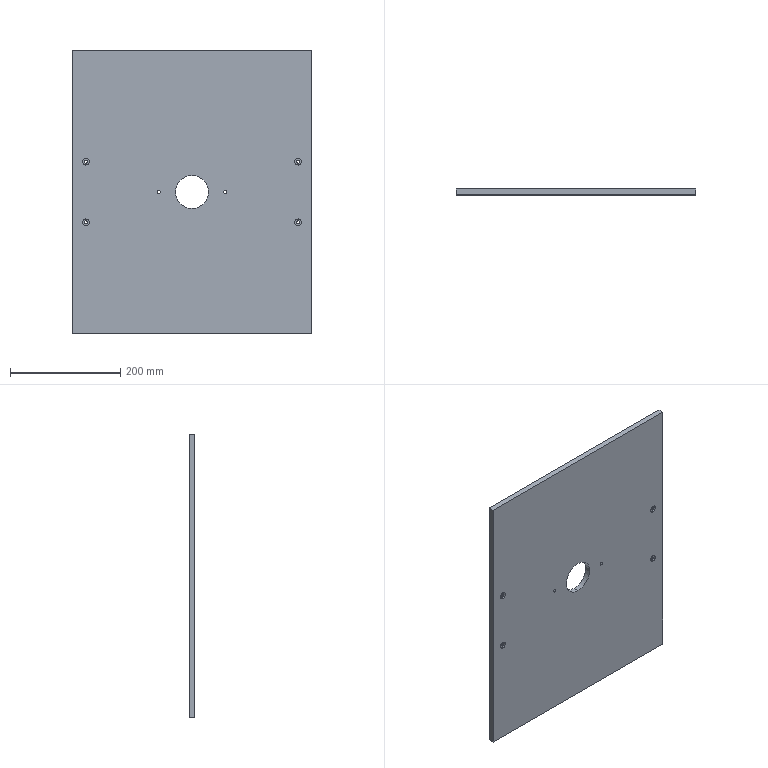Part | SolidWorks | features ICE 2, Extrusion 1, HoleWzd 1 | 1 solid | 40 faces | box 435 x 10 x 515 mm | volume 2209236 mm3 | cylinder 22 | plane 10 | cone 8 | commonest cylinder face diameters 5.5 x12 12.238 x8 60 x2
STEP:
#1=CARTESIAN_POINT('',(192.5,0.025,-48.881));
#2=VERTEX_POINT('',#1);
#3=CARTESIAN_POINT('',(192.5,0.025,-61.119));
#4=VERTEX_POINT('',#3);
#5=CARTESIAN_POINT('',(192.5,0.025,-55.));
#6=DIRECTION('',(0.,-1.,0.));
#7=DIRECTION('',(0.,0.,-1.));
#8=AXIS2_PLACEMENT_3D('',#5,#6,#7);
#9=CIRCLE('',#8,6.119);
#10=EDGE_CURVE('',#2,#4,#9,.T.);
#11=ORIENTED_EDGE('',*,*,#10,.F.);
#12=CARTESIAN_POINT('',(192.5,0.,-48.856));
#13=VERTEX_POINT('',#12);
#14=CARTESIAN_POINT('',(192.5,0.,-48.856));
#15=DIRECTION('',(0.,-0.7071,0.7071));
#16=VECTOR('',#15,1000.);
#17=LINE('',#14,#16);
#18=EDGE_CURVE('',#2,#13,#17,.T.);
#19=ORIENTED_EDGE('',*,*,#18,.T.);
#20=CARTESIAN_POINT('',(192.5,0.,-61.144));
#21=VERTEX_POINT('',#20);
#22=CARTESIAN_POINT('',(192.5,0.,-55.));
#23=DIRECTION('',(0.,-1.,0.));
#24=DIRECTION('',(0.,0.,-1.));
#25=AXIS2_PLACEMENT_3D('',#22,#23,#24);
#26=CIRCLE('',#25,6.144);
#27=EDGE_CURVE('',#13,#21,#26,.T.);
#28=ORIENTED_EDGE('',*,*,#27,.T.);
#29=CARTESIAN_POINT('',(192.5,0.,-61.144));
#30=DIRECTION('',(0.,-0.7071,-0.7071));
#31=VECTOR('',#30,1000.);
#32=LINE('',#29,#31);
#33=EDGE_CURVE('',#4,#21,#32,.T.);
#34=ORIENTED_EDGE('',*,*,#33,.F.);
#35=EDGE_LOOP('',(#11,#19,#28,#34));
#36=FACE_OUTER_BOUND('',#35,.T.);
#37=CARTESIAN_POINT('',(192.5,0.,-55.));
#38=DIRECTION('',(0.,-1.,0.));
#39=DIRECTION('',(0.,0.,-1.));
#40=AXIS2_PLACEMENT_3D('',#37,#38,#39);
#41=CONICAL_SURFACE('',#40,6.144,0.7854);
#42=ADVANCED_FACE('',(#36),#41,.F.);
#43=CARTESIAN_POINT('',(192.5,3.5,-48.881));
#44=VERTEX_POINT('',#43);
#45=CARTESIAN_POINT('',(192.5,3.5,-61.119));
#46=VERTEX_POINT('',#45);
#47=CARTESIAN_POINT('',(192.5,3.5,-55.));
#48=DIRECTION('',(0.,-1.,0.));
#49=DIRECTION('',(0.,0.,-1.));
#50=AXIS2_PLACEMENT_3D('',#47,#48,#49);
#51=CIRCLE('',#50,6.119);
#52=EDGE_CURVE('',#44,#46,#51,.T.);
#53=ORIENTED_EDGE('',*,*,#52,.F.);
#54=CARTESIAN_POINT('',(192.5,0.,-48.881));
#55=DIRECTION('',(0.,-1.,0.));
#56=VECTOR('',#55,1000.);
#57=LINE('',#54,#56);
#58=EDGE_CURVE('',#44,#2,#57,.T.);
#59=ORIENTED_EDGE('',*,*,#58,.T.);
#60=ORIENTED_EDGE('',*,*,#10,.T.);
#61=CARTESIAN_POINT('',(192.5,0.,-61.119));
#62=DIRECTION('',(0.,-1.,0.));
#63=VECTOR('',#62,1000.);
#64=LINE('',#61,#63);
#65=EDGE_CURVE('',#46,#4,#64,.T.);
#66=ORIENTED_EDGE('',*,*,#65,.F.);
#67=EDGE_LOOP('',(#53,#59,#60,#66));
#68=FACE_OUTER_BOUND('',#67,.T.);
#69=CARTESIAN_POINT('',(192.5,0.,-55.));
#70=DIRECTION('',(0.,-1.,0.));
#71=DIRECTION('',(0.,0.,-1.));
#72=AXIS2_PLACEMENT_3D('',#69,#70,#71);
#73=CYLINDRICAL_SURFACE('',#72,6.119);
#74=ADVANCED_FACE('',(#68),#73,.F.);
#75=CARTESIAN_POINT('',(192.5,10.,-52.25));
#76=VERTEX_POINT('',#75);
#77=CARTESIAN_POINT('',(192.5,10.,-57.75));
#78=VERTEX_POINT('',#77);
#79=CARTESIAN_POINT('',(192.5,10.,-55.));
#80=DIRECTION('',(0.,-1.,0.));
#81=DIRECTION('',(0.,0.,-1.));
#82=AXIS2_PLACEMENT_3D('',#79,#80,#81);
#83=CIRCLE('',#82,2.75);
#84=EDGE_CURVE('',#76,#78,#83,.T.);
#85=ORIENTED_EDGE('',*,*,#84,.F.);
#86=CARTESIAN_POINT('',(192.5,3.5,-52.25));
#87=VERTEX_POINT('',#86);
#88=CARTESIAN_POINT('',(192.5,0.,-52.25));
#89=DIRECTION('',(0.,-1.,0.));
#90=VECTOR('',#89,1000.);
#91=LINE('',#88,#90);
#92=EDGE_CURVE('',#76,#87,#91,.T.);
#93=ORIENTED_EDGE('',*,*,#92,.T.);
#94=CARTESIAN_POINT('',(192.5,3.5,-57.75));
#95=VERTEX_POINT('',#94);
#96=CARTESIAN_POINT('',(192.5,3.5,-55.));
#97=DIRECTION('',(0.,-1.,0.));
#98=DIRECTION('',(0.,0.,-1.));
#99=AXIS2_PLACEMENT_3D('',#96,#97,#98);
#100=CIRCLE('',#99,2.75);
#101=EDGE_CURVE('',#87,#95,#100,.T.);
#102=ORIENTED_EDGE('',*,*,#101,.T.);
#103=CARTESIAN_POINT('',(192.5,0.,-57.75));
#104=DIRECTION('',(0.,-1.,0.));
#105=VECTOR('',#104,1000.);
#106=LINE('',#103,#105);
#107=EDGE_CURVE('',#78,#95,#106,.T.);
#108=ORIENTED_EDGE('',*,*,#107,.F.);
#109=EDGE_LOOP('',(#85,#93,#102,#108));
#110=FACE_OUTER_BOUND('',#109,.T.);
#111=CARTESIAN_POINT('',(192.5,0.,-55.));
#112=DIRECTION('',(0.,-1.,0.));
#113=DIRECTION('',(0.,0.,-1.));
#114=AXIS2_PLACEMENT_3D('',#111,#112,#113);
#115=CYLINDRICAL_SURFACE('',#114,2.75);
#116=ADVANCED_FACE('',(#110),#115,.F.);
#117=CARTESIAN_POINT('',(192.5,0.025,61.119));
#118=VERTEX_POINT('',#117);
#119=CARTESIAN_POINT('',(192.5,0.025,48.881));
#120=VERTEX_POINT('',#119);
#121=CARTESIAN_POINT('',(192.5,0.025,55.));
#122=DIRECTION('',(0.,-1.,0.));
#123=DIRECTION('',(0.,0.,-1.));
#124=AXIS2_PLACEMENT_3D('',#121,#122,#123);
#125=CIRCLE('',#124,6.119);
#126=EDGE_CURVE('',#118,#120,#125,.T.);
#127=ORIENTED_EDGE('',*,*,#126,.F.);
#128=CARTESIAN_POINT('',(192.5,0.,61.144));
#129=VERTEX_POINT('',#128);
#130=CARTESIAN_POINT('',(192.5,0.,61.144));
#131=DIRECTION('',(0.,-0.7071,0.7071));
#132=VECTOR('',#131,1000.);
#133=LINE('',#130,#132);
#134=EDGE_CURVE('',#118,#129,#133,.T.);
#135=ORIENTED_EDGE('',*,*,#134,.T.);
#136=CARTESIAN_POINT('',(192.5,0.,48.856));
#137=VERTEX_POINT('',#136);
#138=CARTESIAN_POINT('',(192.5,0.,55.));
#139=DIRECTION('',(0.,-1.,0.));
#140=DIRECTION('',(0.,0.,-1.));
#141=AXIS2_PLACEMENT_3D('',#138,#139,#140);
#142=CIRCLE('',#141,6.144);
#143=EDGE_CURVE('',#129,#137,#142,.T.);
#144=ORIENTED_EDGE('',*,*,#143,.T.);
#145=CARTESIAN_POINT('',(192.5,0.,48.856));
#146=DIRECTION('',(0.,-0.7071,-0.7071));
#147=VECTOR('',#146,1000.);
#148=LINE('',#145,#147);
#149=EDGE_CURVE('',#120,#137,#148,.T.);
#150=ORIENTED_EDGE('',*,*,#149,.F.);
#151=EDGE_LOOP('',(#127,#135,#144,#150));
#152=FACE_OUTER_BOUND('',#151,.T.);
#153=CARTESIAN_POINT('',(192.5,0.,55.));
#154=DIRECTION('',(0.,-1.,0.));
#155=DIRECTION('',(0.,0.,-1.));
#156=AXIS2_PLACEMENT_3D('',#153,#154,#155);
#157=CONICAL_SURFACE('',#156,6.144,0.7854);
#158=ADVANCED_FACE('',(#152),#157,.F.);
#159=CARTESIAN_POINT('',(192.5,3.5,61.119));
#160=VERTEX_POINT('',#159);
#161=CARTESIAN_POINT('',(192.5,3.5,48.881));
#162=VERTEX_POINT('',#161);
#163=CARTESIAN_POINT('',(192.5,3.5,55.));
#164=DIRECTION('',(0.,-1.,0.));
#165=DIRECTION('',(0.,0.,-1.));
#166=AXIS2_PLACEMENT_3D('',#163,#164,#165);
#167=CIRCLE('',#166,6.119);
#168=EDGE_CURVE('',#160,#162,#167,.T.);
#169=ORIENTED_EDGE('',*,*,#168,.F.);
#170=CARTESIAN_POINT('',(192.5,0.,61.119));
#171=DIRECTION('',(0.,-1.,0.));
#172=VECTOR('',#171,1000.);
#173=LINE('',#170,#172);
#174=EDGE_CURVE('',#160,#118,#173,.T.);
#175=ORIENTED_EDGE('',*,*,#174,.T.);
#176=ORIENTED_EDGE('',*,*,#126,.T.);
#177=CARTESIAN_POINT('',(192.5,0.,48.881));
#178=DIRECTION('',(0.,-1.,0.));
#179=VECTOR('',#178,1000.);
#180=LINE('',#177,#179);
#181=EDGE_CURVE('',#162,#120,#180,.T.);
#182=ORIENTED_EDGE('',*,*,#181,.F.);
#183=EDGE_LOOP('',(#169,#175,#176,#182));
#184=FACE_OUTER_BOUND('',#183,.T.);
#185=CARTESIAN_POINT('',(192.5,0.,55.));
#186=DIRECTION('',(0.,-1.,0.));
#187=DIRECTION('',(0.,0.,-1.));
#188=AXIS2_PLACEMENT_3D('',#185,#186,#187);
#189=CYLINDRICAL_SURFACE('',#188,6.119);
#190=ADVANCED_FACE('',(#184),#189,.F.);
#191=CARTESIAN_POINT('',(192.5,10.,57.75));
#192=VERTEX_POINT('',#191);
#193=CARTESIAN_POINT('',(192.5,10.,52.25));
#194=VERTEX_POINT('',#193);
#195=CARTESIAN_POINT('',(192.5,10.,55.));
#196=DIRECTION('',(0.,-1.,0.));
#197=DIRECTION('',(0.,0.,-1.));
#198=AXIS2_PLACEMENT_3D('',#195,#196,#197);
#199=CIRCLE('',#198,2.75);
#200=EDGE_CURVE('',#192,#194,#199,.T.);
#201=ORIENTED_EDGE('',*,*,#200,.F.);
#202=CARTESIAN_POINT('',(192.5,3.5,57.75));
#203=VERTEX_POINT('',#202);
#204=CARTESIAN_POINT('',(192.5,0.,57.75));
#205=DIRECTION('',(0.,-1.,0.));
#206=VECTOR('',#205,1000.);
#207=LINE('',#204,#206);
#208=EDGE_CURVE('',#192,#203,#207,.T.);
#209=ORIENTED_EDGE('',*,*,#208,.T.);
#210=CARTESIAN_POINT('',(192.5,3.5,52.25));
#211=VERTEX_POINT('',#210);
#212=CARTESIAN_POINT('',(192.5,3.5,55.));
#213=DIRECTION('',(0.,-1.,0.));
#214=DIRECTION('',(0.,0.,-1.));
#215=AXIS2_PLACEMENT_3D('',#212,#213,#214);
#216=CIRCLE('',#215,2.75);
#217=EDGE_CURVE('',#203,#211,#216,.T.);
#218=ORIENTED_EDGE('',*,*,#217,.T.);
#219=CARTESIAN_POINT('',(192.5,0.,52.25));
#220=DIRECTION('',(0.,-1.,0.));
#221=VECTOR('',#220,1000.);
#222=LINE('',#219,#221);
#223=EDGE_CURVE('',#194,#211,#222,.T.);
#224=ORIENTED_EDGE('',*,*,#223,.F.);
#225=EDGE_LOOP('',(#201,#209,#218,#224));
#226=FACE_OUTER_BOUND('',#225,.T.);
#227=CARTESIAN_POINT('',(192.5,0.,55.));
#228=DIRECTION('',(0.,-1.,0.));
#229=DIRECTION('',(0.,0.,-1.));
#230=AXIS2_PLACEMENT_3D('',#227,#228,#229);
#231=CYLINDRICAL_SURFACE('',#230,2.75);
#232=ADVANCED_FACE('',(#226),#231,.F.);
#233=CARTESIAN_POINT('',(-192.5,0.025,61.119));
#234=VERTEX_POINT('',#233);
#235=CARTESIAN_POINT('',(-192.5,0.025,48.881));
#236=VERTEX_POINT('',#235);
#237=CARTESIAN_POINT('',(-192.5,0.025,55.));
#238=DIRECTION('',(0.,-1.,0.));
#239=DIRECTION('',(0.,0.,-1.));
#240=AXIS2_PLACEMENT_3D('',#237,#238,#239);
#241=CIRCLE('',#240,6.119);
#242=EDGE_CURVE('',#234,#236,#241,.T.);
#243=ORIENTED_EDGE('',*,*,#242,.F.);
#244=CARTESIAN_POINT('',(-192.5,0.,61.144));
#245=VERTEX_POINT('',#244);
#246=CARTESIAN_POINT('',(-192.5,0.,61.144));
#247=DIRECTION('',(0.,-0.7071,0.7071));
#248=VECTOR('',#247,1000.);
#249=LINE('',#246,#248);
#250=EDGE_CURVE('',#234,#245,#249,.T.);
#251=ORIENTED_EDGE('',*,*,#250,.T.);
#252=CARTESIAN_POINT('',(-192.5,0.,48.856));
#253=VERTEX_POINT('',#252);
#254=CARTESIAN_POINT('',(-192.5,0.,55.));
#255=DIRECTION('',(0.,-1.,0.));
#256=DIRECTION('',(0.,0.,-1.));
#257=AXIS2_PLACEMENT_3D('',#254,#255,#256);
#258=CIRCLE('',#257,6.144);
#259=EDGE_CURVE('',#245,#253,#258,.T.);
#260=ORIENTED_EDGE('',*,*,#259,.T.);
#261=CARTESIAN_POINT('',(-192.5,0.,48.856));
#262=DIRECTION('',(0.,-0.7071,-0.7071));
#263=VECTOR('',#262,1000.);
#264=LINE('',#261,#263);
#265=EDGE_CURVE('',#236,#253,#264,.T.);
#266=ORIENTED_EDGE('',*,*,#265,.F.);
#267=EDGE_LOOP('',(#243,#251,#260,#266));
#268=FACE_OUTER_BOUND('',#267,.T.);
#269=CARTESIAN_POINT('',(-192.5,0.,55.));
#270=DIRECTION('',(0.,-1.,0.));
#271=DIRECTION('',(0.,0.,-1.));
#272=AXIS2_PLACEMENT_3D('',#269,#270,#271);
#273=CONICAL_SURFACE('',#272,6.144,0.7854);
#274=ADVANCED_FACE('',(#268),#273,.F.);
#275=CARTESIAN_POINT('',(-192.5,3.5,61.119));
#276=VERTEX_POINT('',#275);
#277=CARTESIAN_POINT('',(-192.5,3.5,48.881));
#278=VERTEX_POINT('',#277);
#279=CARTESIAN_POINT('',(-192.5,3.5,55.));
#280=DIRECTION('',(0.,-1.,0.));
#281=DIRECTION('',(0.,0.,-1.));
#282=AXIS2_PLACEMENT_3D('',#279,#280,#281);
#283=CIRCLE('',#282,6.119);
#284=EDGE_CURVE('',#276,#278,#283,.T.);
#285=ORIENTED_EDGE('',*,*,#284,.F.);
#286=CARTESIAN_POINT('',(-192.5,0.,61.119));
#287=DIRECTION('',(0.,-1.,0.));
#288=VECTOR('',#287,1000.);
#289=LINE('',#286,#288);
#290=EDGE_CURVE('',#276,#234,#289,.T.);
#291=ORIENTED_EDGE('',*,*,#290,.T.);
#292=ORIENTED_EDGE('',*,*,#242,.T.);
#293=CARTESIAN_POINT('',(-192.5,0.,48.881));
#294=DIRECTION('',(0.,-1.,0.));
#295=VECTOR('',#294,1000.);
#296=LINE('',#293,#295);
#297=EDGE_CURVE('',#278,#236,#296,.T.);
#298=ORIENTED_EDGE('',*,*,#297,.F.);
#299=EDGE_LOOP('',(#285,#291,#292,#298));
#300=FACE_OUTER_BOUND('',#299,.T.);
#301=CARTESIAN_POINT('',(-192.5,0.,55.));
#302=DIRECTION('',(0.,-1.,0.));
#303=DIRECTION('',(0.,0.,-1.));
#304=AXIS2_PLACEMENT_3D('',#301,#302,#303);
#305=CYLINDRICAL_SURFACE('',#304,6.119);
#306=ADVANCED_FACE('',(#300),#305,.F.);
#307=CARTESIAN_POINT('',(-192.5,10.,57.75));
#308=VERTEX_POINT('',#307);
#309=CARTESIAN_POINT('',(-192.5,10.,52.25));
#310=VERTEX_POINT('',#309);
#311=CARTESIAN_POINT('',(-192.5,10.,55.));
#312=DIRECTION('',(0.,-1.,0.));
#313=DIRECTION('',(0.,0.,-1.));
#314=AXIS2_PLACEMENT_3D('',#311,#312,#313);
#315=CIRCLE('',#314,2.75);
#316=EDGE_CURVE('',#308,#310,#315,.T.);
#317=ORIENTED_EDGE('',*,*,#316,.F.);
#318=CARTESIAN_POINT('',(-192.5,3.5,57.75));
#319=VERTEX_POINT('',#318);
#320=CARTESIAN_POINT('',(-192.5,0.,57.75));
#321=DIRECTION('',(0.,-1.,0.));
#322=VECTOR('',#321,1000.);
#323=LINE('',#320,#322);
#324=EDGE_CURVE('',#308,#319,#323,.T.);
#325=ORIENTED_EDGE('',*,*,#324,.T.);
#326=CARTESIAN_POINT('',(-192.5,3.5,52.25));
#327=VERTEX_POINT('',#326);
#328=CARTESIAN_POINT('',(-192.5,3.5,55.));
#329=DIRECTION('',(0.,-1.,0.));
#330=DIRECTION('',(0.,0.,-1.));
#331=AXIS2_PLACEMENT_3D('',#328,#329,#330);
#332=CIRCLE('',#331,2.75);
#333=EDGE_CURVE('',#319,#327,#332,.T.);
#334=ORIENTED_EDGE('',*,*,#333,.T.);
#335=CARTESIAN_POINT('',(-192.5,0.,52.25));
#336=DIRECTION('',(0.,-1.,0.));
#337=VECTOR('',#336,1000.);
#338=LINE('',#335,#337);
#339=EDGE_CURVE('',#310,#327,#338,.T.);
#340=ORIENTED_EDGE('',*,*,#339,.F.);
#341=EDGE_LOOP('',(#317,#325,#334,#340));
#342=FACE_OUTER_BOUND('',#341,.T.);
#343=CARTESIAN_POINT('',(-192.5,0.,55.));
#344=DIRECTION('',(0.,-1.,0.));
#345=DIRECTION('',(0.,0.,-1.));
#346=AXIS2_PLACEMENT_3D('',#343,#344,#345);
#347=CYLINDRICAL_SURFACE('',#346,2.75);
#348=ADVANCED_FACE('',(#342),#347,.F.);
#349=CARTESIAN_POINT('',(-192.5,0.025,-48.881));
#350=VERTEX_POINT('',#349);
#351=CARTESIAN_POINT('',(-192.5,0.025,-61.119));
#352=VERTEX_POINT('',#351);
#353=CARTESIAN_POINT('',(-192.5,0.025,-55.));
#354=DIRECTION('',(0.,-1.,0.));
#355=DIRECTION('',(0.,0.,-1.));
#356=AXIS2_PLACEMENT_3D('',#353,#354,#355);
#357=CIRCLE('',#356,6.119);
#358=EDGE_CURVE('',#350,#352,#357,.T.);
#359=ORIENTED_EDGE('',*,*,#358,.F.);
#360=CARTESIAN_POINT('',(-192.5,0.,-48.856));
#361=VERTEX_POINT('',#360);
#362=CARTESIAN_POINT('',(-192.5,0.,-48.856));
#363=DIRECTION('',(0.,-0.7071,0.7071));
#364=VECTOR('',#363,1000.);
#365=LINE('',#362,#364);
#366=EDGE_CURVE('',#350,#361,#365,.T.);
#367=ORIENTED_EDGE('',*,*,#366,.T.);
#368=CARTESIAN_POINT('',(-192.5,0.,-61.144));
#369=VERTEX_POINT('',#368);
#370=CARTESIAN_POINT('',(-192.5,0.,-55.));
#371=DIRECTION('',(0.,-1.,0.));
#372=DIRECTION('',(0.,0.,-1.));
#373=AXIS2_PLACEMENT_3D('',#370,#371,#372);
#374=CIRCLE('',#373,6.144);
#375=EDGE_CURVE('',#361,#369,#374,.T.);
#376=ORIENTED_EDGE('',*,*,#375,.T.);
#377=CARTESIAN_POINT('',(-192.5,0.,-61.144));
#378=DIRECTION('',(0.,-0.7071,-0.7071));
#379=VECTOR('',#378,1000.);
#380=LINE('',#377,#379);
#381=EDGE_CURVE('',#352,#369,#380,.T.);
#382=ORIENTED_EDGE('',*,*,#381,.F.);
#383=EDGE_LOOP('',(#359,#367,#376,#382));
#384=FACE_OUTER_BOUND('',#383,.T.);
#385=CARTESIAN_POINT('',(-192.5,0.,-55.));
#386=DIRECTION('',(0.,-1.,0.));
#387=DIRECTION('',(0.,0.,-1.));
#388=AXIS2_PLACEMENT_3D('',#385,#386,#387);
#389=CONICAL_SURFACE('',#388,6.144,0.7854);
#390=ADVANCED_FACE('',(#384),#389,.F.);
#391=CARTESIAN_POINT('',(-192.5,3.5,-48.881));
#392=VERTEX_POINT('',#391);
#393=CARTESIAN_POINT('',(-192.5,3.5,-61.119));
#394=VERTEX_POINT('',#393);
#395=CARTESIAN_POINT('',(-192.5,3.5,-55.));
#396=DIRECTION('',(0.,-1.,0.));
#397=DIRECTION('',(0.,0.,-1.));
#398=AXIS2_PLACEMENT_3D('',#395,#396,#397);
#399=CIRCLE('',#398,6.119);
#400=EDGE_CURVE('',#392,#394,#399,.T.);
#401=ORIENTED_EDGE('',*,*,#400,.F.);
#402=CARTESIAN_POINT('',(-192.5,0.,-48.881));
#403=DIRECTION('',(0.,-1.,0.));
#404=VECTOR('',#403,1000.);
#405=LINE('',#402,#404);
#406=EDGE_CURVE('',#392,#350,#405,.T.);
#407=ORIENTED_EDGE('',*,*,#406,.T.);
#408=ORIENTED_EDGE('',*,*,#358,.T.);
#409=CARTESIAN_POINT('',(-192.5,0.,-61.119));
#410=DIRECTION('',(0.,-1.,0.));
#411=VECTOR('',#410,1000.);
#412=LINE('',#409,#411);
#413=EDGE_CURVE('',#394,#352,#412,.T.);
#414=ORIENTED_EDGE('',*,*,#413,.F.);
#415=EDGE_LOOP('',(#401,#407,#408,#414));
#416=FACE_OUTER_BOUND('',#415,.T.);
#417=CARTESIAN_POINT('',(-192.5,0.,-55.));
#418=DIRECTION('',(0.,-1.,0.));
#419=DIRECTION('',(0.,0.,-1.));
#420=AXIS2_PLACEMENT_3D('',#417,#418,#419);
#421=CYLINDRICAL_SURFACE('',#420,6.119);
#422=ADVANCED_FACE('',(#416),#421,.F.);
#423=CARTESIAN_POINT('',(-192.5,10.,-52.25));
#424=VERTEX_POINT('',#423);
#425=CARTESIAN_POINT('',(-192.5,10.,-57.75));
#426=VERTEX_POINT('',#425);
#427=CARTESIAN_POINT('',(-192.5,10.,-55.));
#428=DIRECTION('',(0.,-1.,0.));
#429=DIRECTION('',(0.,0.,-1.));
#430=AXIS2_PLACEMENT_3D('',#427,#428,#429);
#431=CIRCLE('',#430,2.75);
#432=EDGE_CURVE('',#424,#426,#431,.T.);
#433=ORIENTED_EDGE('',*,*,#432,.F.);
#434=CARTESIAN_POINT('',(-192.5,3.5,-52.25));
#435=VERTEX_POINT('',#434);
#436=CARTESIAN_POINT('',(-192.5,0.,-52.25));
#437=DIRECTION('',(0.,-1.,0.));
#438=VECTOR('',#437,1000.);
#439=LINE('',#436,#438);
#440=EDGE_CURVE('',#424,#435,#439,.T.);
#441=ORIENTED_EDGE('',*,*,#440,.T.);
#442=CARTESIAN_POINT('',(-192.5,3.5,-57.75));
#443=VERTEX_POINT('',#442);
#444=CARTESIAN_POINT('',(-192.5,3.5,-55.));
#445=DIRECTION('',(0.,-1.,0.));
#446=DIRECTION('',(0.,0.,-1.));
#447=AXIS2_PLACEMENT_3D('',#444,#445,#446);
#448=CIRCLE('',#447,2.75);
#449=EDGE_CURVE('',#435,#443,#448,.T.);
#450=ORIENTED_EDGE('',*,*,#449,.T.);
#451=CARTESIAN_POINT('',(-192.5,0.,-57.75));
#452=DIRECTION('',(0.,-1.,0.));
#453=VECTOR('',#452,1000.);
#454=LINE('',#451,#453);
#455=EDGE_CURVE('',#426,#443,#454,.T.);
#456=ORIENTED_EDGE('',*,*,#455,.F.);
#457=EDGE_LOOP('',(#433,#441,#450,#456));
#458=FACE_OUTER_BOUND('',#457,.T.);
#459=CARTESIAN_POINT('',(-192.5,0.,-55.));
#460=DIRECTION('',(0.,-1.,0.));
#461=DIRECTION('',(0.,0.,-1.));
#462=AXIS2_PLACEMENT_3D('',#459,#460,#461);
#463=CYLINDRICAL_SURFACE('',#462,2.75);
#464=ADVANCED_FACE('',(#458),#463,.F.);
#465=CARTESIAN_POINT('',(-60.,0.,-2.75));
#466=VERTEX_POINT('',#465);
#467=CARTESIAN_POINT('',(-60.,0.,2.75));
#468=VERTEX_POINT('',#467);
#469=CARTESIAN_POINT('',(-60.,0.,0.));
#470=DIRECTION('',(0.,1.,0.));
#471=DIRECTION('',(0.,0.,1.));
#472=AXIS2_PLACEMENT_3D('',#469,#470,#471);
#473=CIRCLE('',#472,2.75);
#474=EDGE_CURVE('',#466,#468,#473,.T.);
#475=ORIENTED_EDGE('',*,*,#474,.F.);
#476=CARTESIAN_POINT('',(-60.,10.,-2.75));
#477=VERTEX_POINT('',#476);
#478=CARTESIAN_POINT('',(-60.,0.,-2.75));
#479=DIRECTION('',(0.,1.,0.));
#480=VECTOR('',#479,1000.);
#481=LINE('',#478,#480);
#482=EDGE_CURVE('',#466,#477,#481,.T.);
#483=ORIENTED_EDGE('',*,*,#482,.T.);
#484=CARTESIAN_POINT('',(-60.,10.,2.75));
#485=VERTEX_POINT('',#484);
#486=CARTESIAN_POINT('',(-60.,10.,0.));
#487=DIRECTION('',(0.,1.,0.));
#488=DIRECTION('',(0.,0.,1.));
#489=AXIS2_PLACEMENT_3D('',#486,#487,#488);
#490=CIRCLE('',#489,2.75);
#491=EDGE_CURVE('',#477,#485,#490,.T.);
#492=ORIENTED_EDGE('',*,*,#491,.T.);
#493=CARTESIAN_POINT('',(-60.,0.,2.75));
#494=DIRECTION('',(0.,1.,0.));
#495=VECTOR('',#494,1000.);
#496=LINE('',#493,#495);
#497=EDGE_CURVE('',#468,#485,#496,.T.);
#498=ORIENTED_EDGE('',*,*,#497,.F.);
#499=EDGE_LOOP('',(#475,#483,#492,#498));
#500=FACE_OUTER_BOUND('',#499,.T.);
#501=CARTESIAN_POINT('',(-60.,0.,0.));
#502=DIRECTION('',(0.,1.,0.));
#503=DIRECTION('',(0.,0.,1.));
#504=AXIS2_PLACEMENT_3D('',#501,#502,#503);
#505=CYLINDRICAL_SURFACE('',#504,2.75);
#506=ADVANCED_FACE('',(#500),#505,.F.);
#507=CARTESIAN_POINT('',(60.,0.,-2.75));
#508=VERTEX_POINT('',#507);
#509=CARTESIAN_POINT('',(60.,0.,2.75));
#510=VERTEX_POINT('',#509);
#511=CARTESIAN_POINT('',(60.,0.,0.));
#512=DIRECTION('',(0.,1.,0.));
#513=DIRECTION('',(0.,0.,1.));
#514=AXIS2_PLACEMENT_3D('',#511,#512,#513);
#515=CIRCLE('',#514,2.75);
#516=EDGE_CURVE('',#508,#510,#515,.T.);
#517=ORIENTED_EDGE('',*,*,#516,.F.);
#518=CARTESIAN_POINT('',(60.,10.,-2.75));
#519=VERTEX_POINT('',#518);
#520=CARTESIAN_POINT('',(60.,0.,-2.75));
#521=DIRECTION('',(0.,1.,0.));
#522=VECTOR('',#521,1000.);
#523=LINE('',#520,#522);
#524=EDGE_CURVE('',#508,#519,#523,.T.);
#525=ORIENTED_EDGE('',*,*,#524,.T.);
#526=CARTESIAN_POINT('',(60.,10.,2.75));
#527=VERTEX_POINT('',#526);
#528=CARTESIAN_POINT('',(60.,10.,0.));
#529=DIRECTION('',(0.,1.,0.));
#530=DIRECTION('',(0.,0.,1.));
#531=AXIS2_PLACEMENT_3D('',#528,#529,#530);
#532=CIRCLE('',#531,2.75);
#533=EDGE_CURVE('',#519,#527,#532,.T.);
#534=ORIENTED_EDGE('',*,*,#533,.T.);
#535=CARTESIAN_POINT('',(60.,0.,2.75));
#536=DIRECTION('',(0.,1.,0.));
#537=VECTOR('',#536,1000.);
#538=LINE('',#535,#537);
#539=EDGE_CURVE('',#510,#527,#538,.T.);
#540=ORIENTED_EDGE('',*,*,#539,.F.);
#541=EDGE_LOOP('',(#517,#525,#534,#540));
#542=FACE_OUTER_BOUND('',#541,.T.);
#543=CARTESIAN_POINT('',(60.,0.,0.));
#544=DIRECTION('',(0.,1.,0.));
#545=DIRECTION('',(0.,0.,1.));
#546=AXIS2_PLACEMENT_3D('',#543,#544,#545);
#547=CYLINDRICAL_SURFACE('',#546,2.75);
#548=ADVANCED_FACE('',(#542),#547,.F.);
#549=CARTESIAN_POINT('',(0.,0.,-30.));
#550=VERTEX_POINT('',#549);
#551=CARTESIAN_POINT('',(0.,0.,30.));
#552=VERTEX_POINT('',#551);
#553=CARTESIAN_POINT('',(0.,0.,0.));
#554=DIRECTION('',(0.,1.,0.));
#555=DIRECTION('',(0.,0.,1.));
#556=AXIS2_PLACEMENT_3D('',#553,#554,#555);
#557=CIRCLE('',#556,30.);
#558=EDGE_CURVE('',#550,#552,#557,.T.);
#559=ORIENTED_EDGE('',*,*,#558,.F.);
#560=CARTESIAN_POINT('',(0.,10.,-30.));
#561=VERTEX_POINT('',#560);
#562=CARTESIAN_POINT('',(0.,0.,-30.));
#563=DIRECTION('',(0.,1.,0.));
#564=VECTOR('',#563,1000.);
#565=LINE('',#562,#564);
#566=EDGE_CURVE('',#550,#561,#565,.T.);
#567=ORIENTED_EDGE('',*,*,#566,.T.);
#568=CARTESIAN_POINT('',(0.,10.,30.));
#569=VERTEX_POINT('',#568);
#570=CARTESIAN_POINT('',(0.,10.,0.));
#571=DIRECTION('',(0.,1.,0.));
#572=DIRECTION('',(0.,0.,1.));
#573=AXIS2_PLACEMENT_3D('',#570,#571,#572);
#574=CIRCLE('',#573,30.);
#575=EDGE_CURVE('',#561,#569,#574,.T.);
#576=ORIENTED_EDGE('',*,*,#575,.T.);
#577=CARTESIAN_POINT('',(0.,0.,30.));
#578=DIRECTION('',(0.,1.,0.));
#579=VECTOR('',#578,1000.);
#580=LINE('',#577,#579);
#581=EDGE_CURVE('',#552,#569,#580,.T.);
#582=ORIENTED_EDGE('',*,*,#581,.F.);
#583=EDGE_LOOP('',(#559,#567,#576,#582));
#584=FACE_OUTER_BOUND('',#583,.T.);
#585=CARTESIAN_POINT('',(0.,0.,0.));
#586=DIRECTION('',(0.,1.,0.));
#587=DIRECTION('',(0.,0.,1.));
#588=AXIS2_PLACEMENT_3D('',#585,#586,#587);
#589=CYLINDRICAL_SURFACE('',#588,30.);
#590=ADVANCED_FACE('',(#584),#589,.F.);
#591=CARTESIAN_POINT('',(217.5,0.,257.5));
#592=VERTEX_POINT('',#591);
#593=CARTESIAN_POINT('',(217.5,0.,-257.5));
#594=VERTEX_POINT('',#593);
#595=CARTESIAN_POINT('',(217.5,0.,257.5));
#596=DIRECTION('',(0.,0.,-1.));
#597=VECTOR('',#596,1000.);
#598=LINE('',#595,#597);
#599=EDGE_CURVE('',#592,#594,#598,.T.);
#600=ORIENTED_EDGE('',*,*,#599,.T.);
#601=CARTESIAN_POINT('',(217.5,10.,-257.5));
#602=VERTEX_POINT('',#601);
#603=CARTESIAN_POINT('',(217.5,10.,-257.5));
#604=DIRECTION('',(0.,-1.,0.));
#605=VECTOR('',#604,1000.);
#606=LINE('',#603,#605);
#607=EDGE_CURVE('',#602,#594,#606,.T.);
#608=ORIENTED_EDGE('',*,*,#607,.F.);
#609=CARTESIAN_POINT('',(217.5,10.,257.5));
#610=VERTEX_POINT('',#609);
#611=CARTESIAN_POINT('',(217.5,10.,257.5));
#612=DIRECTION('',(0.,0.,-1.));
#613=VECTOR('',#612,1000.);
#614=LINE('',#611,#613);
#615=EDGE_CURVE('',#610,#602,#614,.T.);
#616=ORIENTED_EDGE('',*,*,#615,.F.);
#617=CARTESIAN_POINT('',(217.5,10.,257.5));
#618=DIRECTION('',(0.,-1.,0.));
#619=VECTOR('',#618,1000.);
#620=LINE('',#617,#619);
#621=EDGE_CURVE('',#610,#592,#620,.T.);
#622=ORIENTED_EDGE('',*,*,#621,.T.);
#623=EDGE_LOOP('',(#600,#608,#616,#622));
#624=FACE_OUTER_BOUND('',#623,.T.);
#625=CARTESIAN_POINT('',(217.5,10.,257.5));
#626=DIRECTION('',(-1.,0.,0.));
#627=DIRECTION('',(0.,0.,1.));
#628=AXIS2_PLACEMENT_3D('',#625,#626,#627);
#629=PLANE('',#628);
#630=ADVANCED_FACE('',(#624),#629,.F.);
#631=CARTESIAN_POINT('',(-217.5,0.,-257.5));
#632=VERTEX_POINT('',#631);
#633=CARTESIAN_POINT('',(-217.5,0.,-257.5));
#634=DIRECTION('',(-1.,0.,0.));
#635=VECTOR('',#634,1000.);
#636=LINE('',#633,#635);
#637=EDGE_CURVE('',#594,#632,#636,.T.);
#638=ORIENTED_EDGE('',*,*,#637,.T.);
#639=CARTESIAN_POINT('',(-217.5,10.,-257.5));
#640=VERTEX_POINT('',#639);
#641=CARTESIAN_POINT('',(-217.5,10.,-257.5));
#642=DIRECTION('',(0.,-1.,0.));
#643=VECTOR('',#642,1000.);
#644=LINE('',#641,#643);
#645=EDGE_CURVE('',#640,#632,#644,.T.);
#646=ORIENTED_EDGE('',*,*,#645,.F.);
#647=CARTESIAN_POINT('',(-217.5,10.,-257.5));
#648=DIRECTION('',(-1.,0.,0.));
#649=VECTOR('',#648,1000.);
#650=LINE('',#647,#649);
#651=EDGE_CURVE('',#602,#640,#650,.T.);
#652=ORIENTED_EDGE('',*,*,#651,.F.);
#653=ORIENTED_EDGE('',*,*,#607,.T.);
#654=EDGE_LOOP('',(#638,#646,#652,#653));
#655=FACE_OUTER_BOUND('',#654,.T.);
#656=CARTESIAN_POINT('',(-217.5,10.,-257.5));
#657=DIRECTION('',(0.,0.,1.));
#658=DIRECTION('',(1.,0.,0.));
#659=AXIS2_PLACEMENT_3D('',#656,#657,#658);
#660=PLANE('',#659);
#661=ADVANCED_FACE('',(#655),#660,.F.);
#662=CARTESIAN_POINT('',(-217.5,0.,257.5));
#663=VERTEX_POINT('',#662);
#664=CARTESIAN_POINT('',(-217.5,0.,257.5));
#665=DIRECTION('',(0.,0.,1.));
#666=VECTOR('',#665,1000.);
#667=LINE('',#664,#666);
#668=EDGE_CURVE('',#632,#663,#667,.T.);
#669=ORIENTED_EDGE('',*,*,#668,.T.);
#670=CARTESIAN_POINT('',(-217.5,10.,257.5));
#671=VERTEX_POINT('',#670);
#672=CARTESIAN_POINT('',(-217.5,10.,257.5));
#673=DIRECTION('',(0.,-1.,0.));
#674=VECTOR('',#673,1000.);
#675=LINE('',#672,#674);
#676=EDGE_CURVE('',#671,#663,#675,.T.);
#677=ORIENTED_EDGE('',*,*,#676,.F.);
#678=CARTESIAN_POINT('',(-217.5,10.,257.5));
#679=DIRECTION('',(0.,0.,1.));
#680=VECTOR('',#679,1000.);
#681=LINE('',#678,#680);
#682=EDGE_CURVE('',#640,#671,#681,.T.);
#683=ORIENTED_EDGE('',*,*,#682,.F.);
#684=ORIENTED_EDGE('',*,*,#645,.T.);
#685=EDGE_LOOP('',(#669,#677,#683,#684));
#686=FACE_OUTER_BOUND('',#685,.T.);
#687=CARTESIAN_POINT('',(-217.5,10.,257.5));
#688=DIRECTION('',(1.,0.,0.));
#689=DIRECTION('',(0.,0.,-1.));
#690=AXIS2_PLACEMENT_3D('',#687,#688,#689);
#691=PLANE('',#690);
#692=ADVANCED_FACE('',(#686),#691,.F.);
#693=CARTESIAN_POINT('',(-217.5,0.,257.5));
#694=DIRECTION('',(1.,0.,0.));
#695=VECTOR('',#694,1000.);
#696=LINE('',#693,#695);
#697=EDGE_CURVE('',#663,#592,#696,.T.);
#698=ORIENTED_EDGE('',*,*,#697,.T.);
#699=ORIENTED_EDGE('',*,*,#621,.F.);
#700=CARTESIAN_POINT('',(-217.5,10.,257.5));
#701=DIRECTION('',(1.,0.,0.));
#702=VECTOR('',#701,1000.);
#703=LINE('',#700,#702);
#704=EDGE_CURVE('',#671,#610,#703,.T.);
#705=ORIENTED_EDGE('',*,*,#704,.F.);
#706=ORIENTED_EDGE('',*,*,#676,.T.);
#707=EDGE_LOOP('',(#698,#699,#705,#706));
#708=FACE_OUTER_BOUND('',#707,.T.);
#709=CARTESIAN_POINT('',(-217.5,10.,257.5));
#710=DIRECTION('',(0.,0.,-1.));
#711=DIRECTION('',(-1.,0.,0.));
#712=AXIS2_PLACEMENT_3D('',#709,#710,#711);
#713=PLANE('',#712);
#714=ADVANCED_FACE('',(#708),#713,.F.);
#715=CARTESIAN_POINT('',(192.5,10.,-55.));
#716=DIRECTION('',(0.,-1.,0.));
#717=DIRECTION('',(0.,0.,-1.));
#718=AXIS2_PLACEMENT_3D('',#715,#716,#717);
#719=CIRCLE('',#718,2.75);
#720=EDGE_CURVE('',#78,#76,#719,.T.);
#721=ORIENTED_EDGE('',*,*,#720,.T.);
#722=ORIENTED_EDGE('',*,*,#84,.T.);
#723=EDGE_LOOP('',(#721,#722));
#724=FACE_BOUND('',#723,.T.);
#725=CARTESIAN_POINT('',(192.5,10.,55.));
#726=DIRECTION('',(0.,-1.,0.));
#727=DIRECTION('',(0.,0.,-1.));
#728=AXIS2_PLACEMENT_3D('',#725,#726,#727);
#729=CIRCLE('',#728,2.75);
#730=EDGE_CURVE('',#194,#192,#729,.T.);
#731=ORIENTED_EDGE('',*,*,#730,.T.);
#732=ORIENTED_EDGE('',*,*,#200,.T.);
#733=EDGE_LOOP('',(#731,#732));
#734=FACE_BOUND('',#733,.T.);
#735=CARTESIAN_POINT('',(-192.5,10.,55.));
#736=DIRECTION('',(0.,-1.,0.));
#737=DIRECTION('',(0.,0.,-1.));
#738=AXIS2_PLACEMENT_3D('',#735,#736,#737);
#739=CIRCLE('',#738,2.75);
#740=EDGE_CURVE('',#310,#308,#739,.T.);
#741=ORIENTED_EDGE('',*,*,#740,.T.);
#742=ORIENTED_EDGE('',*,*,#316,.T.);
#743=EDGE_LOOP('',(#741,#742));
#744=FACE_BOUND('',#743,.T.);
#745=CARTESIAN_POINT('',(-192.5,10.,-55.));
#746=DIRECTION('',(0.,-1.,0.));
#747=DIRECTION('',(0.,0.,-1.));
#748=AXIS2_PLACEMENT_3D('',#745,#746,#747);
#749=CIRCLE('',#748,2.75);
#750=EDGE_CURVE('',#426,#424,#749,.T.);
#751=ORIENTED_EDGE('',*,*,#750,.T.);
#752=ORIENTED_EDGE('',*,*,#432,.T.);
#753=EDGE_LOOP('',(#751,#752));
#754=FACE_BOUND('',#753,.T.);
#755=CARTESIAN_POINT('',(-60.,10.,0.));
#756=DIRECTION('',(0.,1.,0.));
#757=DIRECTION('',(0.,0.,1.));
#758=AXIS2_PLACEMENT_3D('',#755,#756,#757);
#759=CIRCLE('',#758,2.75);
#760=EDGE_CURVE('',#485,#477,#759,.T.);
#761=ORIENTED_EDGE('',*,*,#760,.F.);
#762=ORIENTED_EDGE('',*,*,#491,.F.);
#763=EDGE_LOOP('',(#761,#762));
#764=FACE_BOUND('',#763,.T.);
#765=CARTESIAN_POINT('',(60.,10.,0.));
#766=DIRECTION('',(0.,1.,0.));
#767=DIRECTION('',(0.,0.,1.));
#768=AXIS2_PLACEMENT_3D('',#765,#766,#767);
#769=CIRCLE('',#768,2.75);
#770=EDGE_CURVE('',#527,#519,#769,.T.);
#771=ORIENTED_EDGE('',*,*,#770,.F.);
#772=ORIENTED_EDGE('',*,*,#533,.F.);
#773=EDGE_LOOP('',(#771,#772));
#774=FACE_BOUND('',#773,.T.);
#775=CARTESIAN_POINT('',(0.,10.,0.));
#776=DIRECTION('',(0.,1.,0.));
#777=DIRECTION('',(0.,0.,1.));
#778=AXIS2_PLACEMENT_3D('',#775,#776,#777);
#779=CIRCLE('',#778,30.);
#780=EDGE_CURVE('',#569,#561,#779,.T.);
#781=ORIENTED_EDGE('',*,*,#780,.F.);
#782=ORIENTED_EDGE('',*,*,#575,.F.);
#783=EDGE_LOOP('',(#781,#782));
#784=FACE_BOUND('',#783,.T.);
#785=ORIENTED_EDGE('',*,*,#615,.T.);
#786=ORIENTED_EDGE('',*,*,#651,.T.);
#787=ORIENTED_EDGE('',*,*,#682,.T.);
#788=ORIENTED_EDGE('',*,*,#704,.T.);
#789=EDGE_LOOP('',(#785,#786,#787,#788));
#790=FACE_OUTER_BOUND('',#789,.T.);
#791=CARTESIAN_POINT('',(0.,10.,0.));
#792=DIRECTION('',(0.,-1.,0.));
#793=DIRECTION('',(0.,0.,-1.));
#794=AXIS2_PLACEMENT_3D('',#791,#792,#793);
#795=PLANE('',#794);
#796=ADVANCED_FACE('',(#724,#734,#744,#754,#764,#774,#784,#790),#795,.F.);
#797=CARTESIAN_POINT('',(192.5,0.,-55.));
#798=DIRECTION('',(0.,-1.,0.));
#799=DIRECTION('',(0.,0.,-1.));
#800=AXIS2_PLACEMENT_3D('',#797,#798,#799);
#801=CIRCLE('',#800,6.144);
#802=EDGE_CURVE('',#21,#13,#801,.T.);
#803=ORIENTED_EDGE('',*,*,#802,.F.);
#804=ORIENTED_EDGE('',*,*,#27,.F.);
#805=EDGE_LOOP('',(#803,#804));
#806=FACE_BOUND('',#805,.T.);
#807=CARTESIAN_POINT('',(192.5,0.,55.));
#808=DIRECTION('',(0.,-1.,0.));
#809=DIRECTION('',(0.,0.,-1.));
#810=AXIS2_PLACEMENT_3D('',#807,#808,#809);
#811=CIRCLE('',#810,6.144);
#812=EDGE_CURVE('',#137,#129,#811,.T.);
#813=ORIENTED_EDGE('',*,*,#812,.F.);
#814=ORIENTED_EDGE('',*,*,#143,.F.);
#815=EDGE_LOOP('',(#813,#814));
#816=FACE_BOUND('',#815,.T.);
#817=CARTESIAN_POINT('',(-192.5,0.,55.));
#818=DIRECTION('',(0.,-1.,0.));
#819=DIRECTION('',(0.,0.,-1.));
#820=AXIS2_PLACEMENT_3D('',#817,#818,#819);
#821=CIRCLE('',#820,6.144);
#822=EDGE_CURVE('',#253,#245,#821,.T.);
#823=ORIENTED_EDGE('',*,*,#822,.F.);
#824=ORIENTED_EDGE('',*,*,#259,.F.);
#825=EDGE_LOOP('',(#823,#824));
#826=FACE_BOUND('',#825,.T.);
#827=CARTESIAN_POINT('',(-192.5,0.,-55.));
#828=DIRECTION('',(0.,-1.,0.));
#829=DIRECTION('',(0.,0.,-1.));
#830=AXIS2_PLACEMENT_3D('',#827,#828,#829);
#831=CIRCLE('',#830,6.144);
#832=EDGE_CURVE('',#369,#361,#831,.T.);
#833=ORIENTED_EDGE('',*,*,#832,.F.);
#834=ORIENTED_EDGE('',*,*,#375,.F.);
#835=EDGE_LOOP('',(#833,#834));
#836=FACE_BOUND('',#835,.T.);
#837=CARTESIAN_POINT('',(-60.,0.,0.));
#838=DIRECTION('',(0.,1.,0.));
#839=DIRECTION('',(0.,0.,1.));
#840=AXIS2_PLACEMENT_3D('',#837,#838,#839);
#841=CIRCLE('',#840,2.75);
#842=EDGE_CURVE('',#468,#466,#841,.T.);
#843=ORIENTED_EDGE('',*,*,#842,.T.);
#844=ORIENTED_EDGE('',*,*,#474,.T.);
#845=EDGE_LOOP('',(#843,#844));
#846=FACE_BOUND('',#845,.T.);
#847=CARTESIAN_POINT('',(60.,0.,0.));
#848=DIRECTION('',(0.,1.,0.));
#849=DIRECTION('',(0.,0.,1.));
#850=AXIS2_PLACEMENT_3D('',#847,#848,#849);
#851=CIRCLE('',#850,2.75);
#852=EDGE_CURVE('',#510,#508,#851,.T.);
#853=ORIENTED_EDGE('',*,*,#852,.T.);
#854=ORIENTED_EDGE('',*,*,#516,.T.);
#855=EDGE_LOOP('',(#853,#854));
#856=FACE_BOUND('',#855,.T.);
#857=CARTESIAN_POINT('',(0.,0.,0.));
#858=DIRECTION('',(0.,1.,0.));
#859=DIRECTION('',(0.,0.,1.));
#860=AXIS2_PLACEMENT_3D('',#857,#858,#859);
#861=CIRCLE('',#860,30.);
#862=EDGE_CURVE('',#552,#550,#861,.T.);
#863=ORIENTED_EDGE('',*,*,#862,.T.);
#864=ORIENTED_EDGE('',*,*,#558,.T.);
#865=EDGE_LOOP('',(#863,#864));
#866=FACE_BOUND('',#865,.T.);
#867=ORIENTED_EDGE('',*,*,#599,.F.);
#868=ORIENTED_EDGE('',*,*,#697,.F.);
#869=ORIENTED_EDGE('',*,*,#668,.F.);
#870=ORIENTED_EDGE('',*,*,#637,.F.);
#871=EDGE_LOOP('',(#867,#868,#869,#870));
#872=FACE_OUTER_BOUND('',#871,.T.);
#873=CARTESIAN_POINT('',(0.,0.,0.));
#874=DIRECTION('',(0.,-1.,0.));
#875=DIRECTION('',(0.,0.,-1.));
#876=AXIS2_PLACEMENT_3D('',#873,#874,#875);
#877=PLANE('',#876);
#878=ADVANCED_FACE('',(#806,#816,#826,#836,#846,#856,#866,#872),#877,.T.);
#879=ORIENTED_EDGE('',*,*,#566,.F.);
#880=ORIENTED_EDGE('',*,*,#862,.F.);
#881=ORIENTED_EDGE('',*,*,#581,.T.);
#882=ORIENTED_EDGE('',*,*,#780,.T.);
#883=EDGE_LOOP('',(#879,#880,#881,#882));
#884=FACE_OUTER_BOUND('',#883,.T.);
#885=CARTESIAN_POINT('',(0.,0.,0.));
#886=DIRECTION('',(0.,1.,0.));
#887=DIRECTION('',(0.,0.,1.));
#888=AXIS2_PLACEMENT_3D('',#885,#886,#887);
#889=CYLINDRICAL_SURFACE('',#888,30.);
#890=ADVANCED_FACE('',(#884),#889,.F.);
#891=ORIENTED_EDGE('',*,*,#524,.F.);
#892=ORIENTED_EDGE('',*,*,#852,.F.);
#893=ORIENTED_EDGE('',*,*,#539,.T.);
#894=ORIENTED_EDGE('',*,*,#770,.T.);
#895=EDGE_LOOP('',(#891,#892,#893,#894));
#896=FACE_OUTER_BOUND('',#895,.T.);
#897=CARTESIAN_POINT('',(60.,0.,0.));
#898=DIRECTION('',(0.,1.,0.));
#899=DIRECTION('',(0.,0.,1.));
#900=AXIS2_PLACEMENT_3D('',#897,#898,#899);
#901=CYLINDRICAL_SURFACE('',#900,2.75);
#902=ADVANCED_FACE('',(#896),#901,.F.);
#903=ORIENTED_EDGE('',*,*,#482,.F.);
#904=ORIENTED_EDGE('',*,*,#842,.F.);
#905=ORIENTED_EDGE('',*,*,#497,.T.);
#906=ORIENTED_EDGE('',*,*,#760,.T.);
#907=EDGE_LOOP('',(#903,#904,#905,#906));
#908=FACE_OUTER_BOUND('',#907,.T.);
#909=CARTESIAN_POINT('',(-60.,0.,0.));
#910=DIRECTION('',(0.,1.,0.));
#911=DIRECTION('',(0.,0.,1.));
#912=AXIS2_PLACEMENT_3D('',#909,#910,#911);
#913=CYLINDRICAL_SURFACE('',#912,2.75);
#914=ADVANCED_FACE('',(#908),#913,.F.);
#915=ORIENTED_EDGE('',*,*,#440,.F.);
#916=ORIENTED_EDGE('',*,*,#750,.F.);
#917=ORIENTED_EDGE('',*,*,#455,.T.);
#918=CARTESIAN_POINT('',(-192.5,3.5,-55.));
#919=DIRECTION('',(0.,-1.,0.));
#920=DIRECTION('',(0.,0.,-1.));
#921=AXIS2_PLACEMENT_3D('',#918,#919,#920);
#922=CIRCLE('',#921,2.75);
#923=EDGE_CURVE('',#443,#435,#922,.T.);
#924=ORIENTED_EDGE('',*,*,#923,.T.);
#925=EDGE_LOOP('',(#915,#916,#917,#924));
#926=FACE_OUTER_BOUND('',#925,.T.);
#927=CARTESIAN_POINT('',(-192.5,0.,-55.));
#928=DIRECTION('',(0.,-1.,0.));
#929=DIRECTION('',(0.,0.,-1.));
#930=AXIS2_PLACEMENT_3D('',#927,#928,#929);
#931=CYLINDRICAL_SURFACE('',#930,2.75);
#932=ADVANCED_FACE('',(#926),#931,.F.);
#933=ORIENTED_EDGE('',*,*,#923,.F.);
#934=ORIENTED_EDGE('',*,*,#449,.F.);
#935=EDGE_LOOP('',(#933,#934));
#936=FACE_BOUND('',#935,.T.);
#937=CARTESIAN_POINT('',(-192.5,3.5,-55.));
#938=DIRECTION('',(0.,-1.,0.));
#939=DIRECTION('',(0.,0.,-1.));
#940=AXIS2_PLACEMENT_3D('',#937,#938,#939);
#941=CIRCLE('',#940,6.119);
#942=EDGE_CURVE('',#394,#392,#941,.T.);
#943=ORIENTED_EDGE('',*,*,#942,.T.);
#944=ORIENTED_EDGE('',*,*,#400,.T.);
#945=EDGE_LOOP('',(#943,#944));
#946=FACE_OUTER_BOUND('',#945,.T.);
#947=CARTESIAN_POINT('',(-189.75,3.5,-55.));
#948=DIRECTION('',(0.,1.,0.));
#949=DIRECTION('',(0.,0.,1.));
#950=AXIS2_PLACEMENT_3D('',#947,#948,#949);
#951=PLANE('',#950);
#952=ADVANCED_FACE('',(#936,#946),#951,.F.);
#953=ORIENTED_EDGE('',*,*,#406,.F.);
#954=ORIENTED_EDGE('',*,*,#942,.F.);
#955=ORIENTED_EDGE('',*,*,#413,.T.);
#956=CARTESIAN_POINT('',(-192.5,0.025,-55.));
#957=DIRECTION('',(0.,-1.,0.));
#958=DIRECTION('',(0.,0.,-1.));
#959=AXIS2_PLACEMENT_3D('',#956,#957,#958);
#960=CIRCLE('',#959,6.119);
#961=EDGE_CURVE('',#352,#350,#960,.T.);
#962=ORIENTED_EDGE('',*,*,#961,.T.);
#963=EDGE_LOOP('',(#953,#954,#955,#962));
#964=FACE_OUTER_BOUND('',#963,.T.);
#965=CARTESIAN_POINT('',(-192.5,0.,-55.));
#966=DIRECTION('',(0.,-1.,0.));
#967=DIRECTION('',(0.,0.,-1.));
#968=AXIS2_PLACEMENT_3D('',#965,#966,#967);
#969=CYLINDRICAL_SURFACE('',#968,6.119);
#970=ADVANCED_FACE('',(#964),#969,.F.);
#971=ORIENTED_EDGE('',*,*,#366,.F.);
#972=ORIENTED_EDGE('',*,*,#961,.F.);
#973=ORIENTED_EDGE('',*,*,#381,.T.);
#974=ORIENTED_EDGE('',*,*,#832,.T.);
#975=EDGE_LOOP('',(#971,#972,#973,#974));
#976=FACE_OUTER_BOUND('',#975,.T.);
#977=CARTESIAN_POINT('',(-192.5,0.,-55.));
#978=DIRECTION('',(0.,-1.,0.));
#979=DIRECTION('',(0.,0.,-1.));
#980=AXIS2_PLACEMENT_3D('',#977,#978,#979);
#981=CONICAL_SURFACE('',#980,6.144,0.7854);
#982=ADVANCED_FACE('',(#976),#981,.F.);
#983=ORIENTED_EDGE('',*,*,#324,.F.);
#984=ORIENTED_EDGE('',*,*,#740,.F.);
#985=ORIENTED_EDGE('',*,*,#339,.T.);
#986=CARTESIAN_POINT('',(-192.5,3.5,55.));
#987=DIRECTION('',(0.,-1.,0.));
#988=DIRECTION('',(0.,0.,-1.));
#989=AXIS2_PLACEMENT_3D('',#986,#987,#988);
#990=CIRCLE('',#989,2.75);
#991=EDGE_CURVE('',#327,#319,#990,.T.);
#992=ORIENTED_EDGE('',*,*,#991,.T.);
#993=EDGE_LOOP('',(#983,#984,#985,#992));
#994=FACE_OUTER_BOUND('',#993,.T.);
#995=CARTESIAN_POINT('',(-192.5,0.,55.));
#996=DIRECTION('',(0.,-1.,0.));
#997=DIRECTION('',(0.,0.,-1.));
#998=AXIS2_PLACEMENT_3D('',#995,#996,#997);
#999=CYLINDRICAL_SURFACE('',#998,2.75);
#1000=ADVANCED_FACE('',(#994),#999,.F.);
#1001=ORIENTED_EDGE('',*,*,#991,.F.);
#1002=ORIENTED_EDGE('',*,*,#333,.F.);
#1003=EDGE_LOOP('',(#1001,#1002));
#1004=FACE_BOUND('',#1003,.T.);
#1005=CARTESIAN_POINT('',(-192.5,3.5,55.));
#1006=DIRECTION('',(0.,-1.,0.));
#1007=DIRECTION('',(0.,0.,-1.));
#1008=AXIS2_PLACEMENT_3D('',#1005,#1006,#1007);
#1009=CIRCLE('',#1008,6.119);
#1010=EDGE_CURVE('',#278,#276,#1009,.T.);
#1011=ORIENTED_EDGE('',*,*,#1010,.T.);
#1012=ORIENTED_EDGE('',*,*,#284,.T.);
#1013=EDGE_LOOP('',(#1011,#1012));
#1014=FACE_OUTER_BOUND('',#1013,.T.);
#1015=CARTESIAN_POINT('',(-189.75,3.5,55.));
#1016=DIRECTION('',(0.,1.,0.));
#1017=DIRECTION('',(0.,0.,1.));
#1018=AXIS2_PLACEMENT_3D('',#1015,#1016,#1017);
#1019=PLANE('',#1018);
#1020=ADVANCED_FACE('',(#1004,#1014),#1019,.F.);
#1021=ORIENTED_EDGE('',*,*,#290,.F.);
#1022=ORIENTED_EDGE('',*,*,#1010,.F.);
#1023=ORIENTED_EDGE('',*,*,#297,.T.);
#1024=CARTESIAN_POINT('',(-192.5,0.025,55.));
#1025=DIRECTION('',(0.,-1.,0.));
#1026=DIRECTION('',(0.,0.,-1.));
#1027=AXIS2_PLACEMENT_3D('',#1024,#1025,#1026);
#1028=CIRCLE('',#1027,6.119);
#1029=EDGE_CURVE('',#236,#234,#1028,.T.);
#1030=ORIENTED_EDGE('',*,*,#1029,.T.);
#1031=EDGE_LOOP('',(#1021,#1022,#1023,#1030));
#1032=FACE_OUTER_BOUND('',#1031,.T.);
#1033=CARTESIAN_POINT('',(-192.5,0.,55.));
#1034=DIRECTION('',(0.,-1.,0.));
#1035=DIRECTION('',(0.,0.,-1.));
#1036=AXIS2_PLACEMENT_3D('',#1033,#1034,#1035);
#1037=CYLINDRICAL_SURFACE('',#1036,6.119);
#1038=ADVANCED_FACE('',(#1032),#1037,.F.);
#1039=ORIENTED_EDGE('',*,*,#250,.F.);
#1040=ORIENTED_EDGE('',*,*,#1029,.F.);
#1041=ORIENTED_EDGE('',*,*,#265,.T.);
#1042=ORIENTED_EDGE('',*,*,#822,.T.);
#1043=EDGE_LOOP('',(#1039,#1040,#1041,#1042));
#1044=FACE_OUTER_BOUND('',#1043,.T.);
#1045=CARTESIAN_POINT('',(-192.5,0.,55.));
#1046=DIRECTION('',(0.,-1.,0.));
#1047=DIRECTION('',(0.,0.,-1.));
#1048=AXIS2_PLACEMENT_3D('',#1045,#1046,#1047);
#1049=CONICAL_SURFACE('',#1048,6.144,0.7854);
#1050=ADVANCED_FACE('',(#1044),#1049,.F.);
#1051=ORIENTED_EDGE('',*,*,#208,.F.);
#1052=ORIENTED_EDGE('',*,*,#730,.F.);
#1053=ORIENTED_EDGE('',*,*,#223,.T.);
#1054=CARTESIAN_POINT('',(192.5,3.5,55.));
#1055=DIRECTION('',(0.,-1.,0.));
#1056=DIRECTION('',(0.,0.,-1.));
#1057=AXIS2_PLACEMENT_3D('',#1054,#1055,#1056);
#1058=CIRCLE('',#1057,2.75);
#1059=EDGE_CURVE('',#211,#203,#1058,.T.);
#1060=ORIENTED_EDGE('',*,*,#1059,.T.);
#1061=EDGE_LOOP('',(#1051,#1052,#1053,#1060));
#1062=FACE_OUTER_BOUND('',#1061,.T.);
#1063=CARTESIAN_POINT('',(192.5,0.,55.));
#1064=DIRECTION('',(0.,-1.,0.));
#1065=DIRECTION('',(0.,0.,-1.));
#1066=AXIS2_PLACEMENT_3D('',#1063,#1064,#1065);
#1067=CYLINDRICAL_SURFACE('',#1066,2.75);
#1068=ADVANCED_FACE('',(#1062),#1067,.F.);
#1069=ORIENTED_EDGE('',*,*,#1059,.F.);
#1070=ORIENTED_EDGE('',*,*,#217,.F.);
#1071=EDGE_LOOP('',(#1069,#1070));
#1072=FACE_BOUND('',#1071,.T.);
#1073=CARTESIAN_POINT('',(192.5,3.5,55.));
#1074=DIRECTION('',(0.,-1.,0.));
#1075=DIRECTION('',(0.,0.,-1.));
#1076=AXIS2_PLACEMENT_3D('',#1073,#1074,#1075);
#1077=CIRCLE('',#1076,6.119);
#1078=EDGE_CURVE('',#162,#160,#1077,.T.);
#1079=ORIENTED_EDGE('',*,*,#1078,.T.);
#1080=ORIENTED_EDGE('',*,*,#168,.T.);
#1081=EDGE_LOOP('',(#1079,#1080));
#1082=FACE_OUTER_BOUND('',#1081,.T.);
#1083=CARTESIAN_POINT('',(195.25,3.5,55.));
#1084=DIRECTION('',(0.,1.,0.));
#1085=DIRECTION('',(0.,0.,1.));
#1086=AXIS2_PLACEMENT_3D('',#1083,#1084,#1085);
#1087=PLANE('',#1086);
#1088=ADVANCED_FACE('',(#1072,#1082),#1087,.F.);
#1089=ORIENTED_EDGE('',*,*,#174,.F.);
#1090=ORIENTED_EDGE('',*,*,#1078,.F.);
#1091=ORIENTED_EDGE('',*,*,#181,.T.);
#1092=CARTESIAN_POINT('',(192.5,0.025,55.));
#1093=DIRECTION('',(0.,-1.,0.));
#1094=DIRECTION('',(0.,0.,-1.));
#1095=AXIS2_PLACEMENT_3D('',#1092,#1093,#1094);
#1096=CIRCLE('',#1095,6.119);
#1097=EDGE_CURVE('',#120,#118,#1096,.T.);
#1098=ORIENTED_EDGE('',*,*,#1097,.T.);
#1099=EDGE_LOOP('',(#1089,#1090,#1091,#1098));
#1100=FACE_OUTER_BOUND('',#1099,.T.);
#1101=CARTESIAN_POINT('',(192.5,0.,55.));
#1102=DIRECTION('',(0.,-1.,0.));
#1103=DIRECTION('',(0.,0.,-1.));
#1104=AXIS2_PLACEMENT_3D('',#1101,#1102,#1103);
#1105=CYLINDRICAL_SURFACE('',#1104,6.119);
#1106=ADVANCED_FACE('',(#1100),#1105,.F.);
#1107=ORIENTED_EDGE('',*,*,#134,.F.);
#1108=ORIENTED_EDGE('',*,*,#1097,.F.);
#1109=ORIENTED_EDGE('',*,*,#149,.T.);
#1110=ORIENTED_EDGE('',*,*,#812,.T.);
#1111=EDGE_LOOP('',(#1107,#1108,#1109,#1110));
#1112=FACE_OUTER_BOUND('',#1111,.T.);
#1113=CARTESIAN_POINT('',(192.5,0.,55.));
#1114=DIRECTION('',(0.,-1.,0.));
#1115=DIRECTION('',(0.,0.,-1.));
#1116=AXIS2_PLACEMENT_3D('',#1113,#1114,#1115);
#1117=CONICAL_SURFACE('',#1116,6.144,0.7854);
#1118=ADVANCED_FACE('',(#1112),#1117,.F.);
#1119=ORIENTED_EDGE('',*,*,#92,.F.);
#1120=ORIENTED_EDGE('',*,*,#720,.F.);
#1121=ORIENTED_EDGE('',*,*,#107,.T.);
#1122=CARTESIAN_POINT('',(192.5,3.5,-55.));
#1123=DIRECTION('',(0.,-1.,0.));
#1124=DIRECTION('',(0.,0.,-1.));
#1125=AXIS2_PLACEMENT_3D('',#1122,#1123,#1124);
#1126=CIRCLE('',#1125,2.75);
#1127=EDGE_CURVE('',#95,#87,#1126,.T.);
#1128=ORIENTED_EDGE('',*,*,#1127,.T.);
#1129=EDGE_LOOP('',(#1119,#1120,#1121,#1128));
#1130=FACE_OUTER_BOUND('',#1129,.T.);
#1131=CARTESIAN_POINT('',(192.5,0.,-55.));
#1132=DIRECTION('',(0.,-1.,0.));
#1133=DIRECTION('',(0.,0.,-1.));
#1134=AXIS2_PLACEMENT_3D('',#1131,#1132,#1133);
#1135=CYLINDRICAL_SURFACE('',#1134,2.75);
#1136=ADVANCED_FACE('',(#1130),#1135,.F.);
#1137=ORIENTED_EDGE('',*,*,#1127,.F.);
#1138=ORIENTED_EDGE('',*,*,#101,.F.);
#1139=EDGE_LOOP('',(#1137,#1138));
#1140=FACE_BOUND('',#1139,.T.);
#1141=CARTESIAN_POINT('',(192.5,3.5,-55.));
#1142=DIRECTION('',(0.,-1.,0.));
#1143=DIRECTION('',(0.,0.,-1.));
#1144=AXIS2_PLACEMENT_3D('',#1141,#1142,#1143);
#1145=CIRCLE('',#1144,6.119);
#1146=EDGE_CURVE('',#46,#44,#1145,.T.);
#1147=ORIENTED_EDGE('',*,*,#1146,.T.);
#1148=ORIENTED_EDGE('',*,*,#52,.T.);
#1149=EDGE_LOOP('',(#1147,#1148));
#1150=FACE_OUTER_BOUND('',#1149,.T.);
#1151=CARTESIAN_POINT('',(195.25,3.5,-55.));
#1152=DIRECTION('',(0.,1.,0.));
#1153=DIRECTION('',(0.,0.,1.));
#1154=AXIS2_PLACEMENT_3D('',#1151,#1152,#1153);
#1155=PLANE('',#1154);
#1156=ADVANCED_FACE('',(#1140,#1150),#1155,.F.);
#1157=ORIENTED_EDGE('',*,*,#58,.F.);
#1158=ORIENTED_EDGE('',*,*,#1146,.F.);
#1159=ORIENTED_EDGE('',*,*,#65,.T.);
#1160=CARTESIAN_POINT('',(192.5,0.025,-55.));
#1161=DIRECTION('',(0.,-1.,0.));
#1162=DIRECTION('',(0.,0.,-1.));
#1163=AXIS2_PLACEMENT_3D('',#1160,#1161,#1162);
#1164=CIRCLE('',#1163,6.119);
#1165=EDGE_CURVE('',#4,#2,#1164,.T.);
#1166=ORIENTED_EDGE('',*,*,#1165,.T.);
#1167=EDGE_LOOP('',(#1157,#1158,#1159,#1166));
#1168=FACE_OUTER_BOUND('',#1167,.T.);
#1169=CARTESIAN_POINT('',(192.5,0.,-55.));
#1170=DIRECTION('',(0.,-1.,0.));
#1171=DIRECTION('',(0.,0.,-1.));
#1172=AXIS2_PLACEMENT_3D('',#1169,#1170,#1171);
#1173=CYLINDRICAL_SURFACE('',#1172,6.119);
#1174=ADVANCED_FACE('',(#1168),#1173,.F.);
#1175=ORIENTED_EDGE('',*,*,#18,.F.);
#1176=ORIENTED_EDGE('',*,*,#1165,.F.);
#1177=ORIENTED_EDGE('',*,*,#33,.T.);
#1178=ORIENTED_EDGE('',*,*,#802,.T.);
#1179=EDGE_LOOP('',(#1175,#1176,#1177,#1178));
#1180=FACE_OUTER_BOUND('',#1179,.T.);
#1181=CARTESIAN_POINT('',(192.5,0.,-55.));
#1182=DIRECTION('',(0.,-1.,0.));
#1183=DIRECTION('',(0.,0.,-1.));
#1184=AXIS2_PLACEMENT_3D('',#1181,#1182,#1183);
#1185=CONICAL_SURFACE('',#1184,6.144,0.7854);
#1186=ADVANCED_FACE('',(#1180),#1185,.F.);
#1187=CLOSED_SHELL('',(#42,#74,#116,#158,#190,#232,#274,#306,#348,#390,#422,#464,#506,#548,#590,#630,#661,#692,#714,#796,#878,#890,#902,#914,#932,#952,#970,#982,#1000,#1020,#1038,#1050,#1068,#1088,#1106,#1118,#1136,#1156,#1174,#1186));
#1188=MANIFOLD_SOLID_BREP('',#1187);
#1189=CARTESIAN_POINT('',(0.,0.,0.));
#1190=DIRECTION('',(0.,0.,1.));
#1191=DIRECTION('',(1.,0.,0.));
#1192=AXIS2_PLACEMENT_3D('',#1189,#1190,#1191);
#1193=(LENGTH_UNIT()NAMED_UNIT(*)SI_UNIT(.MILLI.,.METRE.));
#1194=UNCERTAINTY_MEASURE_WITH_UNIT(LENGTH_MEASURE(0.00001),#1193,'','');
#1195=(NAMED_UNIT(*)PLANE_ANGLE_UNIT()SI_UNIT($,.RADIAN.));
#1196=(NAMED_UNIT(*)SI_UNIT($,.STERADIAN.)SOLID_ANGLE_UNIT());
#1197=(GEOMETRIC_REPRESENTATION_CONTEXT(3)GLOBAL_UNCERTAINTY_ASSIGNED_CONTEXT((#1194))GLOBAL_UNIT_ASSIGNED_CONTEXT((#1193,#1195,#1196))REPRESENTATION_CONTEXT('',''));
#1198=ADVANCED_BREP_SHAPE_REPRESENTATION('',(#1188,#1192),#1197);